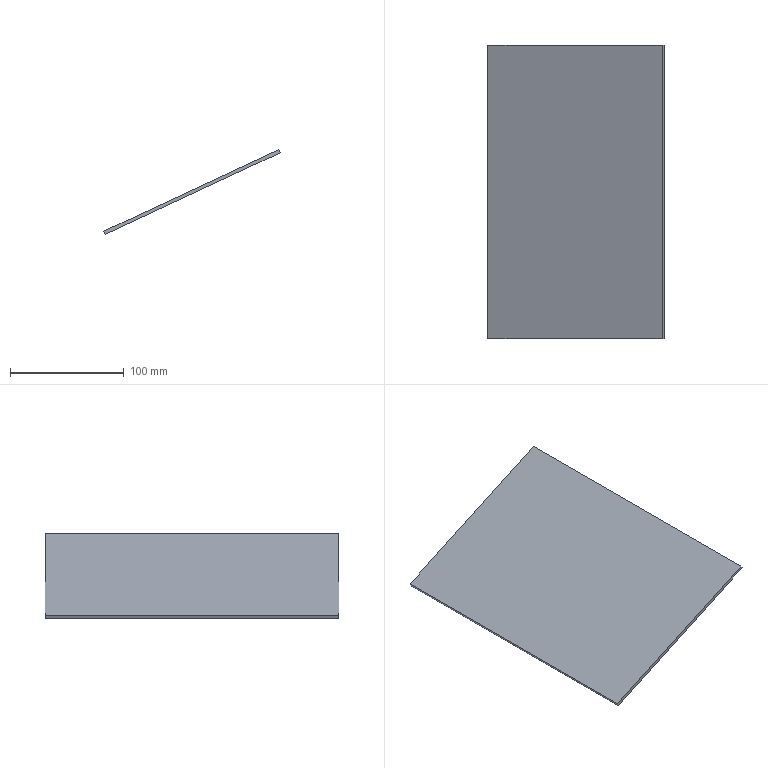Part | NX | features solid 2 | 1 solid | 6 faces | box 154.905 x 258 x 74.361 mm | volume 131208 mm3 | plane 6
STEP:
#1=CARTESIAN_POINT('',(-239.369,320.,-179.361));
#2=VERTEX_POINT('',#1);
#3=CARTESIAN_POINT('',(-240.637,320.,-176.642));
#4=VERTEX_POINT('',#3);
#5=CARTESIAN_POINT('',(-240.637,320.,-176.642));
#6=DIRECTION('',(-0.4226,0.,0.9063));
#7=VECTOR('',#6,1000.);
#8=LINE('',#5,#7);
#9=EDGE_CURVE('',#2,#4,#8,.T.);
#10=ORIENTED_EDGE('',*,*,#9,.T.);
#11=CARTESIAN_POINT('',(-87.,320.,-105.));
#12=VERTEX_POINT('',#11);
#13=CARTESIAN_POINT('',(-87.,320.,-105.));
#14=DIRECTION('',(-0.9063,0.,-0.4226));
#15=VECTOR('',#14,1000.);
#16=LINE('',#13,#15);
#17=EDGE_CURVE('',#12,#4,#16,.T.);
#18=ORIENTED_EDGE('',*,*,#17,.F.);
#19=CARTESIAN_POINT('',(-85.732,320.,-107.719));
#20=VERTEX_POINT('',#19);
#21=CARTESIAN_POINT('',(-87.,320.,-105.));
#22=DIRECTION('',(-0.4226,0.,0.9063));
#23=VECTOR('',#22,1000.);
#24=LINE('',#21,#23);
#25=EDGE_CURVE('',#20,#12,#24,.T.);
#26=ORIENTED_EDGE('',*,*,#25,.F.);
#27=CARTESIAN_POINT('',(-85.732,320.,-107.719));
#28=DIRECTION('',(0.9063,0.,0.4226));
#29=VECTOR('',#28,1000.);
#30=LINE('',#27,#29);
#31=EDGE_CURVE('',#20,#2,#30,.F.);
#32=ORIENTED_EDGE('',*,*,#31,.T.);
#33=EDGE_LOOP('',(#10,#18,#26,#32));
#34=FACE_BOUND('',#33,.T.);
#35=CARTESIAN_POINT('',(-87.,320.,-105.));
#36=DIRECTION('',(0.,1.,0.));
#37=DIRECTION('',(-0.9063,0.,-0.4226));
#38=AXIS2_PLACEMENT_3D('',#35,#36,#37);
#39=PLANE('',#38);
#40=ADVANCED_FACE('',(#34),#39,.T.);
#41=ORIENTED_EDGE('',*,*,#25,.T.);
#42=CARTESIAN_POINT('',(-87.,62.,-105.));
#43=VERTEX_POINT('',#42);
#44=CARTESIAN_POINT('',(-87.,320.,-105.));
#45=DIRECTION('',(0.,-1.,0.));
#46=VECTOR('',#45,1000.);
#47=LINE('',#44,#46);
#48=EDGE_CURVE('',#12,#43,#47,.T.);
#49=ORIENTED_EDGE('',*,*,#48,.T.);
#50=CARTESIAN_POINT('',(-85.732,62.,-107.719));
#51=VERTEX_POINT('',#50);
#52=CARTESIAN_POINT('',(-87.,62.,-105.));
#53=DIRECTION('',(-0.4226,0.,0.9063));
#54=VECTOR('',#53,1000.);
#55=LINE('',#52,#54);
#56=EDGE_CURVE('',#51,#43,#55,.T.);
#57=ORIENTED_EDGE('',*,*,#56,.F.);
#58=CARTESIAN_POINT('',(-85.732,320.,-107.719));
#59=DIRECTION('',(0.,1.,0.));
#60=VECTOR('',#59,1000.);
#61=LINE('',#58,#60);
#62=EDGE_CURVE('',#20,#51,#61,.F.);
#63=ORIENTED_EDGE('',*,*,#62,.F.);
#64=EDGE_LOOP('',(#41,#49,#57,#63));
#65=FACE_BOUND('',#64,.T.);
#66=CARTESIAN_POINT('',(-87.,320.,-105.));
#67=DIRECTION('',(-0.9063,0.,-0.4226));
#68=DIRECTION('',(0.,-1.,0.));
#69=AXIS2_PLACEMENT_3D('',#66,#67,#68);
#70=PLANE('',#69);
#71=ADVANCED_FACE('',(#65),#70,.F.);
#72=ORIENTED_EDGE('',*,*,#56,.T.);
#73=CARTESIAN_POINT('',(-240.637,62.,-176.642));
#74=VERTEX_POINT('',#73);
#75=CARTESIAN_POINT('',(-52.135,62.,-88.742));
#76=DIRECTION('',(0.9063,0.,0.4226));
#77=VECTOR('',#76,1000.);
#78=LINE('',#75,#77);
#79=EDGE_CURVE('',#43,#74,#78,.F.);
#80=ORIENTED_EDGE('',*,*,#79,.T.);
#81=CARTESIAN_POINT('',(-239.369,62.,-179.361));
#82=VERTEX_POINT('',#81);
#83=CARTESIAN_POINT('',(-283.502,62.,-84.719));
#84=DIRECTION('',(0.4226,0.,-0.9063));
#85=VECTOR('',#84,1000.);
#86=LINE('',#83,#85);
#87=EDGE_CURVE('',#82,#74,#86,.F.);
#88=ORIENTED_EDGE('',*,*,#87,.F.);
#89=CARTESIAN_POINT('',(-50.867,62.,-91.461));
#90=DIRECTION('',(0.9063,0.,0.4226));
#91=VECTOR('',#90,1000.);
#92=LINE('',#89,#91);
#93=EDGE_CURVE('',#51,#82,#92,.F.);
#94=ORIENTED_EDGE('',*,*,#93,.F.);
#95=EDGE_LOOP('',(#72,#80,#88,#94));
#96=FACE_BOUND('',#95,.T.);
#97=CARTESIAN_POINT('',(-95.,62.,3.181));
#98=DIRECTION('',(0.,1.,0.));
#99=DIRECTION('',(-1.,0.,0.));
#100=AXIS2_PLACEMENT_3D('',#97,#98,#99);
#101=PLANE('',#100);
#102=ADVANCED_FACE('',(#96),#101,.F.);
#103=CARTESIAN_POINT('',(-239.369,320.,-179.361));
#104=DIRECTION('',(0.,1.,0.));
#105=VECTOR('',#104,1000.);
#106=LINE('',#103,#105);
#107=EDGE_CURVE('',#2,#82,#106,.F.);
#108=ORIENTED_EDGE('',*,*,#107,.T.);
#109=ORIENTED_EDGE('',*,*,#87,.T.);
#110=CARTESIAN_POINT('',(-240.637,320.,-176.642));
#111=DIRECTION('',(0.,-1.,0.));
#112=VECTOR('',#111,1000.);
#113=LINE('',#110,#112);
#114=EDGE_CURVE('',#4,#74,#113,.T.);
#115=ORIENTED_EDGE('',*,*,#114,.F.);
#116=ORIENTED_EDGE('',*,*,#9,.F.);
#117=EDGE_LOOP('',(#108,#109,#115,#116));
#118=FACE_BOUND('',#117,.T.);
#119=CARTESIAN_POINT('',(-240.637,320.,-176.642));
#120=DIRECTION('',(-0.9063,0.,-0.4226));
#121=DIRECTION('',(0.,-1.,0.));
#122=AXIS2_PLACEMENT_3D('',#119,#120,#121);
#123=PLANE('',#122);
#124=ADVANCED_FACE('',(#118),#123,.T.);
#125=ORIENTED_EDGE('',*,*,#79,.F.);
#126=ORIENTED_EDGE('',*,*,#48,.F.);
#127=ORIENTED_EDGE('',*,*,#17,.T.);
#128=ORIENTED_EDGE('',*,*,#114,.T.);
#129=EDGE_LOOP('',(#125,#126,#127,#128));
#130=FACE_BOUND('',#129,.T.);
#131=CARTESIAN_POINT('',(-87.,320.,-105.));
#132=DIRECTION('',(0.4226,0.,-0.9063));
#133=DIRECTION('',(0.9063,0.,0.4226));
#134=AXIS2_PLACEMENT_3D('',#131,#132,#133);
#135=PLANE('',#134);
#136=ADVANCED_FACE('',(#130),#135,.F.);
#137=ORIENTED_EDGE('',*,*,#93,.T.);
#138=ORIENTED_EDGE('',*,*,#107,.F.);
#139=ORIENTED_EDGE('',*,*,#31,.F.);
#140=ORIENTED_EDGE('',*,*,#62,.T.);
#141=EDGE_LOOP('',(#137,#138,#139,#140));
#142=FACE_BOUND('',#141,.T.);
#143=CARTESIAN_POINT('',(-85.732,320.,-107.719));
#144=DIRECTION('',(0.4226,0.,-0.9063));
#145=DIRECTION('',(0.9063,0.,0.4226));
#146=AXIS2_PLACEMENT_3D('',#143,#144,#145);
#147=PLANE('',#146);
#148=ADVANCED_FACE('',(#142),#147,.T.);
#149=CLOSED_SHELL('',(#40,#71,#102,#124,#136,#148));
#150=MANIFOLD_SOLID_BREP('',#149);
#151=(LENGTH_UNIT()NAMED_UNIT(*)SI_UNIT(.MILLI.,.METRE.));
#152=UNCERTAINTY_MEASURE_WITH_UNIT(LENGTH_MEASURE(0.00001),#151,'','');
#153=(NAMED_UNIT(*)PLANE_ANGLE_UNIT()SI_UNIT($,.RADIAN.));
#154=(NAMED_UNIT(*)SI_UNIT($,.STERADIAN.)SOLID_ANGLE_UNIT());
#155=(GEOMETRIC_REPRESENTATION_CONTEXT(3)GLOBAL_UNCERTAINTY_ASSIGNED_CONTEXT((#152))GLOBAL_UNIT_ASSIGNED_CONTEXT((#151,#153,#154))REPRESENTATION_CONTEXT('',''));
#156=ADVANCED_BREP_SHAPE_REPRESENTATION('',(#150),#155);